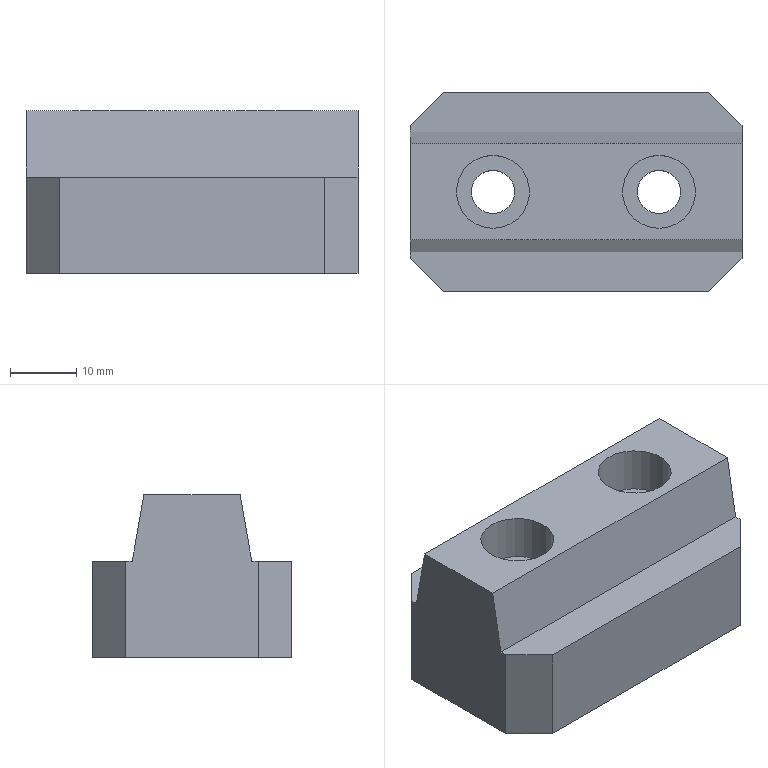Part | STEP file | solid 103 | 1 solid | 20 faces | box 50 x 30 x 24.5 mm | volume 26652 mm3 | plane 16 | cylinder 4 | commonest cylinder face diameters 6.5 x2 11 x2